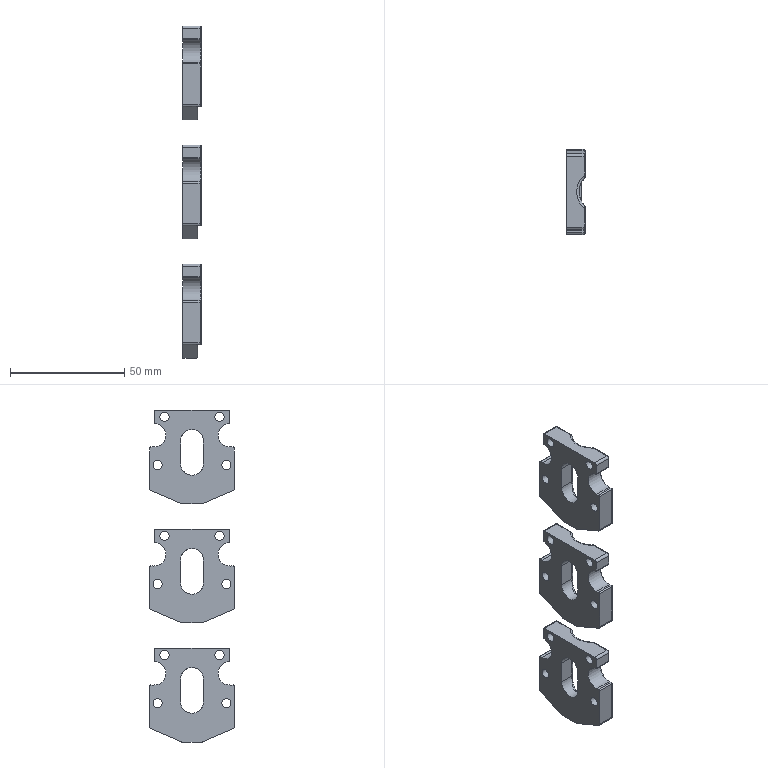Part | 3 solids | 321 faces | box 8 x 37 x 145 mm | volume 23104 mm3 | cylinder 141 | plane 57 | spline 54 | torus 51 | sphere 18 | commonest cylinder face diameters 1 x63 2 x24 4 x18 0.4 x15 10 x6 10.3 x6